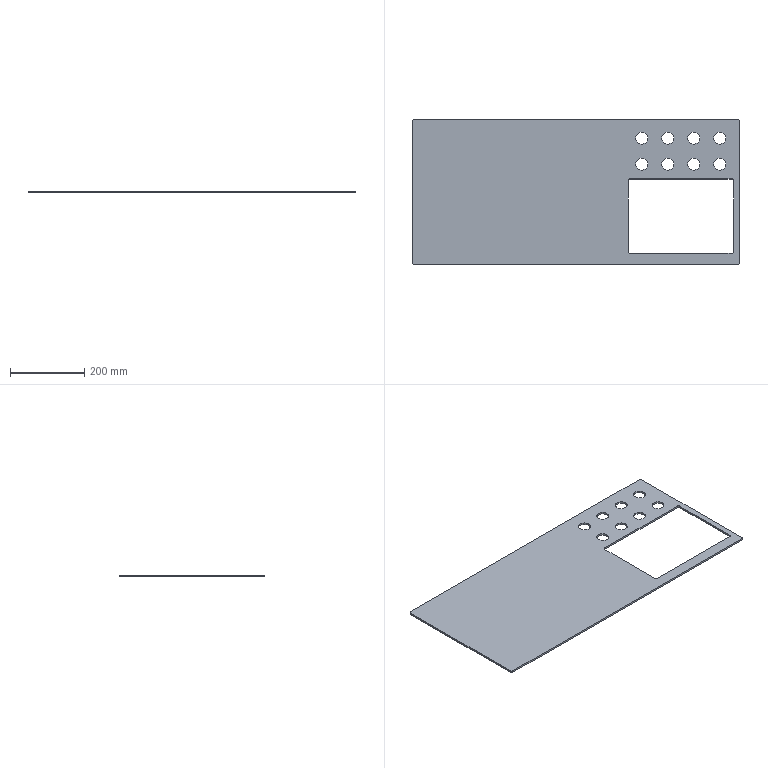Part | STEP file | 001-002-Face Plate-6 | 1 solid | 34 faces | box 880 x 390 x 5 mm | volume 1398830 mm3 | cylinder 24 | plane 10 | commonest cylinder face diameters 32 x16 10 x8